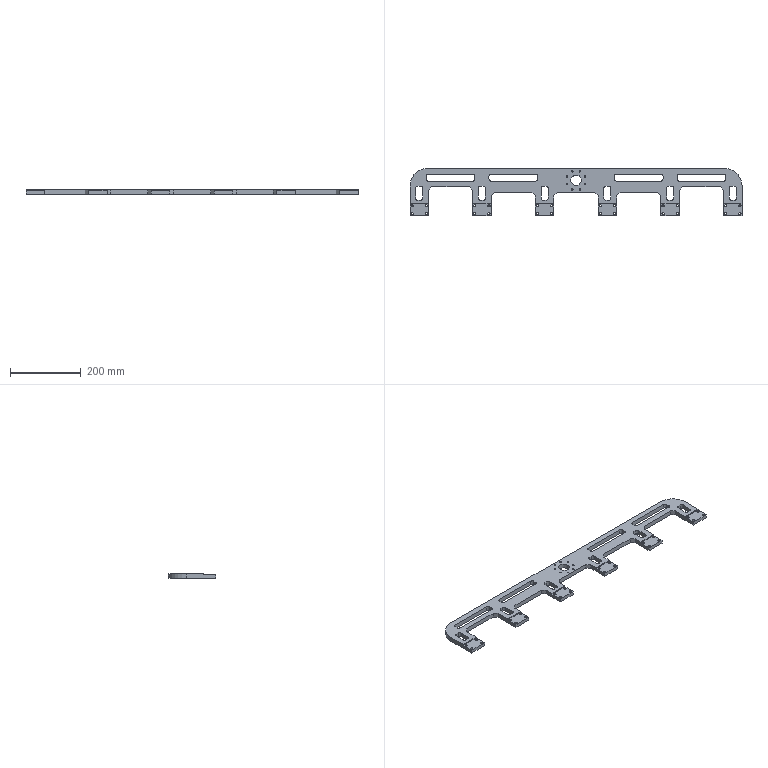NC program | NX | posted with a generic post | part box 941 x 134 x 13 mm
Lines 1 to 72 of 4152:
N10 G17 G21 G94 G90
(FLOOR_WALL_COPY_COPY , TOOL : D63)
N12 T01 M6
N14 G54
N16 G17 G0 G90 X507. Y-68.997 S6500 M3
N18 G43 Z30. H1
N20 Z3.
N22 G94 G1 Z0. F1500.
N24 X504.
N26 X53.089
N28 Y-40.798
N30 X504.
N32 Y-12.599
N34 X53.089
N36 Y15.601
N38 X504.
N40 Y43.8
N42 X53.089
N44 Y71.999
N46 X504.
N48 X507.
N50 Z3.
N52 G0 Z30.
N54 M5
(DRILLING_COPY_1_COPY , TOOL : D6A45)
N56 T07 M6
N58 G54
N60 G17 G0 G90 X464.5 Y-39.2 S5000 M3
N62 G43 Z30. H7
N64 G94 G81 G98 Z-1. F250. R3.
N66 Y-61.2
N68 X424.5
N70 Y-39.2
N72 X286.7 Y-61.2
N74 Y-39.2
N76 X246.7
N78 Y-61.2
N80 X108.9
N82 Y-39.2
N84 X68.9
N86 Y-61.2
N88 G80
N90 G0 X68.9 Y-61.2 Z30.
N92 M5
(DRILLING_COPY_COPY_COPY_COPY , TOOL : 6.5ZT)
N94 T15 M6
N96 G54
N98 G17 G0 G90 X464.5 Y-39.2 S2000 M3
N100 G43 Z30. H15
N102 G94 G83 G98 Z-15.953 F250. Q2. R3.
N104 Y-61.2
N106 X424.5
N108 Y-39.2
N110 X286.7 Y-61.2
N112 Y-39.2
N114 X246.7
N116 Y-61.2
N118 X108.9
N120 Y-39.2
N122 X68.9
N124 Y-61.2
N126 G80
N128 G0 X68.9 Y-61.2 Z30.
N130 M5